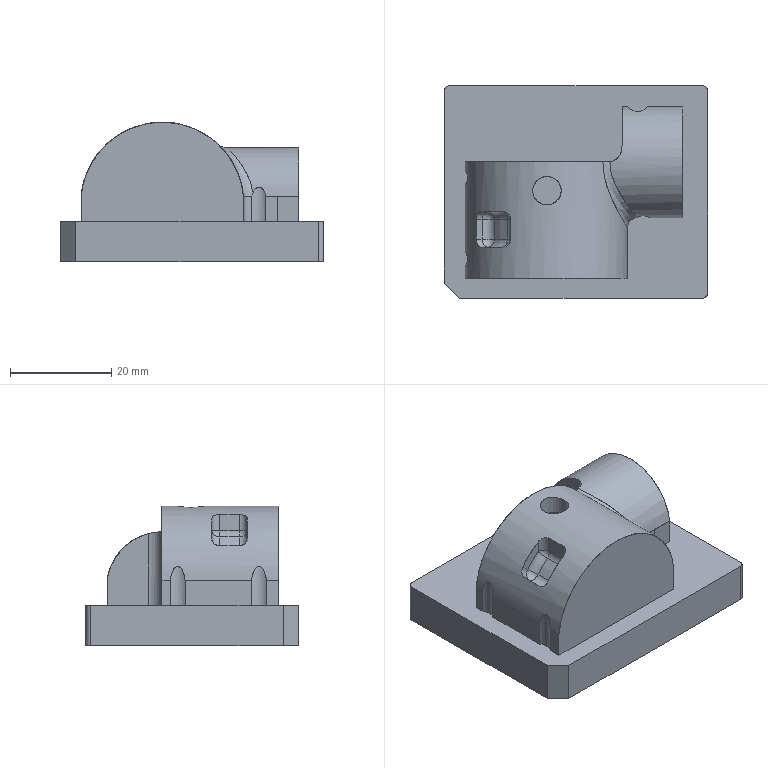NC program | PowerMill | posted with a generic post | part box 52 x 42 x 27.622 mm
Lines 34978 to 35880 of 322299:
N35075 M6
N35076 S8500 M03
N35077 G00 G90 X0.0 Y0.0
N35078 G43 Z9.8022 H3
N35079
N35080 G05 P10000 R8
N35081 X-31.8487 Y-27.3606
N35082 Z-18.62
N35083 G01 Z-19.82 F360.0
N35084 X-28.1181 Y-23.6313 F600.0
N35085 X-25.6571 Y-21.0381
N35086 X-25.7337 Y-20.9654
N35087 X-25.9275 Y-20.7611
N35088 G02 X-26.2819 Y-20.3235 I4.7332 J4.1953
N35089 G01 X-26.4415 Y-20.0914
N35090 X-26.5886 Y-19.8512
N35091 X-26.723 Y-19.6037
N35092 X-26.8443 Y-19.3494
N35093 X-26.9521 Y-19.0892
N35094 X-27.0461 Y-18.8237
N35095 X-27.1261 Y-18.5536
N35096 X-27.1919 Y-18.2798
N35097 X-27.2432 Y-18.0028
N35098 X-27.28 Y-17.7236
N35099 X-27.3021 Y-17.4428
N35100 X-27.3094 Y-17.1612
N35101 Y-14.7229
N35102 X-27.3036 Y-14.4732
N35103 X-27.2863 Y-14.2241
N35104 G02 X-27.2169 Y-13.7296 I6.013 J-0.5908
N35105 G01 X-27.1651 Y-13.4853
N35106 G03 Y-13.002 I-0.9704 J0.2416
N35107 G01 X-27.2169 Y-12.7577
N35108 G02 X-27.2836 Y-12.2858 I5.5385 J1.0235
N35109 G01 X-27.3036 Y-12.0141
N35110 X-27.3094 Y-11.7644
N35111 Y1.3491
N35112 X-27.3036 Y1.5988
N35113 X-27.2863 Y1.8479
N35114 X-27.2573 Y2.096
N35115 X-27.2169 Y2.3424
N35116 X-27.1652 Y2.5867
N35117 G03 X-27.1651 Y3.07 I-0.9703 J0.2417
N35118 G01 X-27.2169 Y3.3143
N35119 X-27.2574 Y3.5607
N35120 X-27.2863 Y3.8088
N35121 X-27.3036 Y4.0579
N35122 X-27.3094 Y4.3076
N35123 Y5.9414
N35124 X-27.3021 Y6.223
N35125 X-27.28 Y6.5038
N35126 X-27.2432 Y6.783
N35127 X-27.1919 Y7.06
N35128 G02 X-27.0461 Y7.6039 I6.0891 J-1.3403
N35129 G01 X-26.9521 Y7.8694
N35130 X-26.8443 Y8.1296
N35131 X-26.723 Y8.3839
N35132 X-26.5886 Y8.6314
N35133 X-26.4415 Y8.8716
N35134 X-26.2819 Y9.1037
N35135 X-26.1105 Y9.3271
N35136 X-25.9275 Y9.5413
N35137 X-25.7337 Y9.7456
N35138 G02 X-25.3152 Y10.1224 I4.4805 J-4.5554
N35139 G01 X-25.0917 Y10.2939
N35140 X-24.939 Y10.3996
N35141 X-24.6194 Y10.6006
N35142 G02 X-24.1177 Y10.8563 I3.1471 J-5.5562
N35143 G02 X-23.6375 Y11.0427 I2.5178 J-5.7736
N35144 G01 X-25.0116 Y15.6429
N35145 X-25.5677 Y15.4768
N35146 G02 X-26.6731 Y16.3431 I-0.2462 J0.8242
N35147 G01 X-26.5211 Y19.4408
N35148 G02 X-24.2089 Y21.645 I2.3149 J-0.1135
N35149 G01 X-1.0643 Y21.6726
N35150 G02 X-0.2545 Y20.5497 I0.001 J-0.8527
N35151 G01 X-0.3586 Y20.2381
N35152 G03 X-0.885 Y18.0053 I11.9898 J-4.0052
N35153 G01 X-0.9904 Y17.2609
N35154 G02 X-2.2961 Y16.1268 I-1.3061 J0.185
N35155 G01 X-21.9374 Y16.1214
N35156 G03 X-24.8262 Y15.6983 I0.0062 J-10.115
N35157 G01 X-25.0116 Y15.6429
N35158 X-23.6375 Y11.0427
N35159 X-23.5919 Y11.0581
N35160 G02 X-23.048 Y11.2038 I1.9409 J-6.1558
N35161 G02 X-22.4918 Y11.2919 I1.2833 J-6.3024
N35162 G02 X-21.9294 Y11.3214 I0.6203 J-6.4566
N35163 G01 X2.7714
N35164 G03 X3.7713 Y12.3039 I0.0 J1.0
N35165 G01 X3.8512 Y16.882
N35166 X3.8633 Y17.1603
N35167 X3.8897 Y17.4376
N35168 X3.9305 Y17.7131
N35169 G02 X4.0545 Y18.256 I6.1181 J-1.112
N35170 G01 X4.1374 Y18.5219
N35171 X4.234 Y18.7832
N35172 X4.3439 Y19.0391
N35173 X4.467 Y19.289
N35174 X4.6028 Y19.5322
N35175 X4.751 Y19.768
N35176 X4.9112 Y19.9958
N35177 X5.083 Y20.2151
N35178 X5.2659 Y20.4251
N35179 G02 X5.6631 Y20.8154 I4.6843 J-4.3696
N35180 G01 X5.8763 Y20.9947
N35181 G02 X6.3292 Y21.3188 I3.9432 J-5.0294
N35182 G02 X6.813 Y21.5945 I3.414 J-5.4309
N35183 G02 X7.3228 Y21.8186 I2.7941 J-5.6635
N35184 G01 X7.5857 Y21.9106
N35185 X7.853 Y21.9888
N35186 X8.124 Y22.0532
N35187 G02 X8.9519 Y22.1609 I1.153 J-5.6244
N35188 G01 X9.2304 Y22.1681
N35189 X10.276
N35190 X10.5574 Y22.1608
N35191 X10.8381 Y22.1387
N35192 X11.1172 Y22.102
N35193 X11.3941 Y22.0507
N35194 X11.6678 Y21.985
N35195 X11.9192 Y21.9105
N35196 G03 X12.4871 I0.284 J0.9589
N35197 G01 X12.7386 Y21.985
N35198 X13.0124 Y22.0507
N35199 G02 X13.5684 Y22.1387 I1.2893 J-6.3441
N35200 G01 X13.849 Y22.1608
N35201 X14.1305 Y22.1681
N35202 X21.0985
N35203 G02 X21.6609 Y22.1387 I-0.0522 J-6.3768
N35204 G01 X21.9401 Y22.1019
N35205 G02 X22.491 Y21.9848 I-1.0667 J-6.3733
N35206 G01 X22.761 Y21.9048
N35207 X23.0265 Y21.8108
N35208 X23.2868 Y21.703
N35209 X23.541 Y21.5818
N35210 X23.7885 Y21.4473
N35211 X24.0287 Y21.3002
N35212 X24.2608 Y21.1406
N35213 X24.4843 Y20.9692
N35214 X24.6984 Y20.7862
N35215 X24.9028 Y20.5924
N35216 X25.0967 Y20.3881
N35217 X25.2796 Y20.1739
N35218 G02 X25.6106 Y19.7183 I-5.0349 J-4.0059
N35219 G01 X25.7578 Y19.4781
N35220 G02 X26.0134 Y18.9764 I-5.3387 J-3.0361
N35221 G01 X26.1212 Y18.7162
N35222 X26.2152 Y18.4506
N35223 X26.2952 Y18.1806
N35224 G02 X26.4123 Y17.6297 I-6.1271 J-1.5904
N35225 G01 X26.4491 Y17.3505
N35226 X26.4712 Y17.0697
N35227 X26.4785 Y16.7881
N35228 Y-5.1044
N35229 X26.4712 Y-5.386
N35230 G02 X26.4123 Y-5.9461 I-6.3455 J0.384
N35231 G01 X26.361 Y-6.223
N35232 X26.2952 Y-6.4969
N35233 G02 X26.1212 Y-7.0325 I-6.0528 J1.6708
N35234 G01 X26.0134 Y-7.2927
N35235 X25.8921 Y-7.5469
N35236 G02 X25.6106 Y-8.0346 I-5.4965 J2.8484
N35237 G01 X25.451 Y-8.2667
N35238 X25.2796 Y-8.4902
N35239 X25.0966 Y-8.7044
N35240 X24.9028 Y-8.9087
N35241 X24.6609 Y-9.1346
N35242 X24.4843 Y-9.2855
N35243 X24.2608 Y-9.457
N35244 X24.0287 Y-9.6165
N35245 G02 X23.541 Y-9.898 I-3.4798 J5.4641
N35246 G01 X23.3637 Y-9.9833
N35247 X23.1837 Y-10.063
N35248 X24.9739 Y-14.5121
N35249 X25.5789 Y-14.2687
N35250 G02 X26.672 Y-15.0123 I0.2972 J-0.7384
N35251 G01 X26.6451 Y-19.12
N35252 G02 X24.1039 Y-21.6553 I-2.5521 J0.0168
N35253 G01 X20.6535 Y-21.6699
N35254 G02 X19.7994 Y-20.5579 I-0.0038 J0.8811
N35255 G01 X20.015 Y-19.7638
N35256 G03 X20.4201 Y-16.8462 I-11.2116 J3.0438
N35257 G01 X20.4236 Y-16.5257
N35258 G02 X21.4806 Y-15.3283 I1.2218 J-0.0133
N35259 G01 X22.4201 Y-15.2004
N35260 G03 X24.8875 Y-14.5469 I-1.3955 J10.2539
N35261 G01 X24.9739 Y-14.5121
N35262 X23.1837 Y-10.063
N35263 X23.0265 Y-10.1271
N35264 G02 X22.491 Y-10.3011 I-2.2591 J6.0418
N35265 G01 X22.2171 Y-10.3669
N35266 G02 X21.6609 Y-10.455 I-1.2851 J6.3138
N35267 G01 X21.3801 Y-10.4771
N35268 X21.0985 Y-10.4844
N35269 X16.5539
N35270 G03 X15.5539 Y-11.4844 I0.0 J-1.0
N35271 G01 Y-17.1612
N35272 G02 X15.5244 Y-17.7236 I-6.4151 J0.0544
N35273 G01 X15.4877 Y-18.0028
N35274 X15.4363 Y-18.2798
N35275 G02 X15.2906 Y-18.8237 I-6.2037 J1.3709
N35276 G01 X15.1966 Y-19.0892
N35277 X15.0888 Y-19.3494
N35278 G02 X14.8331 Y-19.8512 I-5.7149 J2.5959
N35279 G01 X14.6859 Y-20.0914
N35280 X14.5264 Y-20.3235
N35281 X14.3549 Y-20.547
N35282 X14.172 Y-20.7611
N35283 X13.9511 Y-20.9911
N35284 X13.7738 Y-21.1593
N35285 X13.5596 Y-21.3423
N35286 X13.3362 Y-21.5137
N35287 G02 X12.8011 Y-21.8545 I-3.2487 J4.5101
N35288 G01 X12.6164 Y-21.9548
N35289 G02 X12.1019 Y-22.1839 I-2.856 J5.7221
N35290 G01 X11.8364 Y-22.2779
N35291 X11.5663 Y-22.3579
N35292 G02 X11.0155 Y-22.475 I-1.6116 J6.2279
N35293 G01 X10.7362 Y-22.5117
N35294 X10.4554 Y-22.5338
N35295 X10.1739 Y-22.5412
N35296 X-21.9294
N35297 X-22.211 Y-22.5338
N35298 X-22.4918 Y-22.5117
N35299 X-22.7711 Y-22.475
N35300 X-23.048 Y-22.4236
N35301 G02 X-23.592 Y-22.2779 I1.3914 J6.2809
N35302 G02 X-24.1177 Y-22.0761 I2.0424 J6.106
N35303 G02 X-24.6194 Y-21.8204 I2.6836 J5.887
N35304 G01 X-24.867 Y-21.6684
N35305 X-25.0917 Y-21.5137
N35306 X-25.3152 Y-21.3422
N35307 X-25.5294 Y-21.1593
N35308 X-25.6571 Y-21.0381
N35309 X-28.1181 Y-23.6313
N35310 G00 Z9.8022
N35311 G05 P0
N35312 (---------------)
N35313 ( END TOOLPATH : 精公基准台01-基准面偏置-D10 )
N35314 (---------------)
N35315 ( START TOOLPATH : 精公基准台01-外形侧光-D10 )
N35316 (---------------)
N35317 G00 X0.0 Y0.0 Z10.802
N35318 G05 P10000 R8
N35319 X-22.6288 Y11.0478
N35320 Z-8.294
N35321 G01 Z-9.494 F360.0
N35322 G03 X-21.4997 Y10.8403 I0.815 J1.2593 F600.0
N35323 G02 X-20.4463 Y10.9514 I1.0491 J-4.899
N35324 G01 X3.9012
N35325 G03 X4.1212 Y11.1676 I0.0 J0.22
N35326 G01 X4.1792 Y14.5154
N35327 G02 X4.3087 Y15.6056 I5.0106 J-0.0423
N35328 G03 X4.1205 Y16.7381 I-1.4612 J0.3391
N35329 G00 Z4.0256
N35330 G01 X26.2065 Y16.6492 F10000.0
N35331 G00 Z-8.294
N35332 G01 Z-9.494 F360.0
N35333 G03 X25.9982 Y15.5203 I1.2587 J-0.8159 F600.0
N35334 G02 X26.1084 Y14.5132 I-4.8997 J-1.0455
N35335 G01 X26.1083 Y-2.8318
N35336 G02 X25.9992 Y-3.832 I-5.01 J0.0407
N35337 G03 X26.2086 Y-4.9608 I1.4672 J-0.3116
N35338 G00 Z4.0256
N35339 G01 X10.8659 Y-22.2707 F10000.0
N35340 G00 Z-8.294
N35341 G01 Z-9.494 F360.0
N35342 G03 X9.7371 Y-22.0616 I-0.8168 J-1.2581 F600.0
N35343 G02 X8.7627 Y-22.1707 I-1.0422 J4.9005
N35344 G01 X-5.9331 Y-22.171
N35345 X-20.4477 Y-22.1712
N35346 G02 X-21.4998 Y-22.0601 I-0.0028 J5.0101
N35347 G03 X-22.629 Y-22.2675 I-0.3142 J-1.4667
N35348 G00 Z4.0256
N35349 G01 X-22.1045 Y11.1586 F10000.0
N35350 G00 Z-8.294
N35351 G01 Z-9.494 F360.0
N35352 G03 X-21.0014 Y10.8405 I0.9355 J1.1725 F600.0
N35353 G02 X-20.4464 Y10.8714 I0.5509 J-4.8994
N35354 G01 X-20.4463
N35355 X3.9012
N35356 G03 X4.2012 Y11.1662 I0.0 J0.3
N35357 G01 X4.2592 Y14.5132
N35358 G02 X4.3 Y15.1075 I4.9305 J-0.0401
N35359 G03 X4.0008 Y16.2159 I-1.4875 J0.193
N35360 G00 Z4.0256
N35361 G01 X26.3175 Y16.1231 F10000.0
N35362 G00 Z-8.294
N35363 G01 Z-9.494 F360.0
N35364 G03 X25.9982 Y15.0203 I1.1715 J-0.9368 F600.0
N35365 G02 X26.0284 Y14.5132 I-4.8991 J-0.5455
N35366 G01 Y-2.8296
N35367 G02 X25.9991 Y-3.3283 I-4.9304 J0.0385
N35368 G03 X26.3203 Y-4.4305 I1.4911 J-0.1635
N35369 G00 Z4.0256
N35370 G01 X10.3369 Y-22.3822 F10000.0
N35371 G00 Z-8.294
N35372 G01 Z-9.494 F360.0
N35373 G03 X9.2345 Y-22.0616 I-0.9382 J-1.1703 F600.0
N35374 G02 X8.7627 Y-22.0907 I-0.5396 J4.9001
N35375 G01 X-5.9331 Y-22.0912
N35376 X-20.4463
N35377 G02 X-21.0034 Y-22.0601 I-0.0042 J4.9299
N35378 G03 X-22.1067 Y-22.3777 I-0.1683 J-1.4905
N35379 G00 Z3.8883
N35380 G01 X15.6233 Y-12.1522 F10000.0
N35381 G00 Z-18.59
N35382 G01 Z-19.79 F360.0
N35383 G03 X15.1839 Y-13.2128 I1.0606 J-1.0606 F600.0
N35384 G01 Y-17.0694
N35385 G02 X10.2232 Y-22.171 I-5.0119 J-0.0892
N35386 G01 X-5.9331 Y-22.1711
N35387 X-21.0034 Y-22.1712
N35388 X-21.9079
N35389 G02 X-26.9386 Y-17.2516 I-0.0214 J5.0101
N35390 G01 X-26.9393 Y-14.6939
N35391 G02 X-26.7343 Y-13.307 I4.93 J-0.0202
N35392 G03 X-26.7338 Y-13.1846 I-0.2111 J0.0622
N35393 G02 X-26.9394 Y-11.7749 I4.7923 J1.419
N35394 G01 Y1.371
N35395 G02 X-26.7342 Y2.7679 I4.9962 J-0.0204
N35396 G03 Y2.8887 I-0.2115 J0.0605
N35397 G02 X-26.9394 Y4.2901 I4.7926 J1.4177
N35398 G01 Y5.9344
N35399 G02 X-21.9068 Y10.9514 I5.0102 J0.0068
N35400 G01 X-20.4464
N35401 X3.9013
N35402 G03 X4.116 Y11.1237 I0.0 J0.22
N35403 G03 X4.1212 Y11.1676 I-0.2148 J0.0477
N35404 G01 X4.2214 Y16.8895
N35405 G02 X9.3104 Y21.7981 I5.011 J-0.1028
N35406 G02 X10.4093 Y21.7964 I0.4565 J-57.2258
N35407 G02 X12.1216 Y21.4452 I-0.123 J-4.9497
N35408 G03 X12.2855 Y21.4447 I0.0826 J0.2039
N35409 G02 X14.0568 Y21.7976 I1.8327 J-4.5763
N35410 G01 X21.1793 Y21.7975
N35411 G02 X26.1085 Y16.7039 I-0.0824 J-5.0116
N35412 G01 Y-5.0207
N35413 G02 X21.1765 Y-10.1138 I-5.0115 J-0.0815
N35414 G01 X15.4039 Y-10.1144
N35415 G03 X15.1839 Y-10.3344 I0.0 J-0.22
N35416 G01 Y-13.2128
N35417 G03 X15.6232 Y-14.2735 I1.5 J0.0
N35418 G01 X15.5433 Y-12.0854
N35419 G03 X15.1039 Y-13.146 I1.0606 J-1.0606
N35420 G01 Y-17.069
N35421 G02 X10.2232 Y-22.091 I-4.9319 J-0.0896
N35422 G01 X-5.9331 Y-22.0912
N35423 X-21.0034
N35424 X-21.9068
N35425 G02 X-26.8586 Y-17.2516 I-0.0225 J4.9301
N35426 G02 X-26.8594 Y-14.6958 I279.1536 J1.3602
N35427 G02 X-26.6576 Y-13.3296 I4.85 J-0.0183
N35428 G03 X-26.6568 Y-13.1627 I-0.2878 J0.0848
N35429 G02 X-26.8594 Y-11.7749 I4.7132 J1.3968
N35430 G01 Y1.3692
N35431 G02 X-26.6573 Y2.7459 I4.9162 J-0.0186
N35432 G03 X-26.6572 Y2.9107 I-0.2884 J0.0825
N35433 G02 X-26.8594 Y4.2901 I4.7139 J1.3954
N35434 G01 Y5.9331
N35435 G02 X-21.9068 Y10.8714 I4.9301 J0.0082
N35436 G01 X-20.4464
N35437 X3.9013
N35438 G03 X4.1941 Y11.1063 I0.0 J0.3
N35439 G03 X4.2012 Y11.1662 I-0.2929 J0.0651
N35440 G01 X4.3013 Y16.8865
N35441 G02 X9.3104 Y21.7181 I4.9311 J-0.0998
N35442 G02 X10.4057 Y21.7164 I0.4564 J-58.6332
N35443 G02 X12.0916 Y21.371 I-0.1194 J-4.8696
N35444 G03 X12.3151 Y21.3703 I0.1126 J0.2781
N35445 G02 X14.0568 Y21.7176 I1.8029 J-4.5009
N35446 G01 X21.1765 Y21.7175
N35447 G02 X26.0285 Y16.7039 I-0.0796 J-4.9316
N35448 G01 Y-5.0203
N35449 G02 X21.1765 Y-10.0338 I-4.9315 J-0.0819
N35450 G01 X15.4039 Y-10.0344
N35451 G03 X15.1039 Y-10.3344 I0.0 J-0.3
N35452 G01 Y-13.146
N35453 G03 X15.5432 Y-14.2067 I1.5 J0.0
N35454 G00 Z10.802
N35455 G05 P0
N35456 (---------------)
N35457 ( END TOOLPATH : 精公基准台01-外形侧光-D10 )
N35458 (---------------)
N35459 ( START TOOLPATH : 精公基准台01-基准台侧光-D10 )
N35460 (---------------)
N35461 G00 X0.0 Y0.0 Z9.8022
N35462 G05 P10000 R8
N35463 X31.3451 Y-29.0791
N35464 Z-26.52
N35465 G01 Z-27.72 F360.0
N35466 G03 X28.4718 Y-24.9872 I-1.4367 J2.0459 F600.0
N35467 G01 X28.341 Y-25.079
N35468 X28.3395 Y-25.0801
N35469 X28.3379 Y-25.0811
N35470 X28.1487 Y-25.2011
N35471 X28.1476 Y-25.2018
N35472 X28.1464 Y-25.2025
N35473 X28.0195 Y-25.2772
N35474 X28.018 Y-25.2781
N35475 X28.0165 Y-25.2789
N35476 X27.7004 Y-25.4474
N35477 X27.6988 Y-25.4482
N35478 X27.6972 Y-25.449
N35479 X27.5446 Y-25.5219
N35480 X27.5435 Y-25.5224
N35481 X27.5424 Y-25.5229
N35482 X27.379 Y-25.5952
N35483 X27.3774 Y-25.5959
N35484 X27.3758 Y-25.5965
N35485 X27.0597 Y-25.7205
N35486 X27.0574 Y-25.7213
N35487 X27.0551 Y-25.7221
N35488 X26.6842 Y-25.842
N35489 X26.6821 Y-25.8426
N35490 X26.68 Y-25.8432
N35491 X26.4186 Y-25.9122
N35492 X26.4166 Y-25.9127
N35493 X26.4146 Y-25.9131
N35494 X26.0984 Y-25.9794
N35495 X26.0965 Y-25.9798
N35496 X26.0945 Y-25.9802
N35497 X25.7783 Y-26.03
N35498 X25.7761 Y-26.0303
N35499 X25.7739 Y-26.0305
N35500 X25.4577 Y-26.0623
N35501 X25.4557 Y-26.0624
N35502 X25.4537 Y-26.0626
N35503 X25.1375 Y-26.0781
N35504 X25.1358 Y-26.0782
N35505 X25.134
N35506 X24.8179 Y-26.08
N35507 X24.8177
N35508 X24.8174
N35509 X-22.9206
N35510 X-22.9213
N35511 X-22.922
N35512 X-23.2381 Y-26.0744
N35513 X-23.2406 Y-26.0743
N35514 X-23.243 Y-26.0742
N35515 X-23.5592 Y-26.0491
N35516 X-23.5617 Y-26.0489
N35517 X-23.5642 Y-26.0485
N35518 X-23.8804 Y-26.0031
N35519 X-23.8829 Y-26.0027
N35520 X-23.8854 Y-26.0022
N35521 X-24.2016 Y-25.9358
N35522 X-24.2041 Y-25.9352
N35523 X-24.2066 Y-25.9346
N35524 X-24.5228 Y-25.8464
N35525 X-24.5253 Y-25.8456
N35526 X-24.5279 Y-25.8448
N35527 X-24.844 Y-25.7335
N35528 X-24.8465 Y-25.7325
N35529 X-24.8491 Y-25.7315
N35530 X-25.1652 Y-25.5954
N35531 X-25.1671 Y-25.5946
N35532 X-25.1689 Y-25.5937
N35533 X-25.3157 Y-25.5215
N35534 X-25.3169 Y-25.5209
N35535 X-25.3182 Y-25.5202
N35536 X-25.4876 Y-25.4293
N35537 X-25.4895 Y-25.4282
N35538 X-25.4915 Y-25.427
N35539 X-25.8076 Y-25.2336
N35540 X-25.8102 Y-25.2319
N35541 X-25.8127 Y-25.2302
N35542 X-26.1288 Y-25.002
N35543 X-26.1307 Y-25.0006
N35544 X-26.1325 Y-24.9992
N35545 X-26.2796 Y-24.8795
N35546 X-26.2809 Y-24.8784
N35547 X-26.2822 Y-24.8773
N35548 X-26.4512 Y-24.7277
N35549 X-26.4525 Y-24.7264
N35550 X-26.4539 Y-24.7252
N35551 X-26.6255 Y-24.5587
N35552 X-26.6259 Y-24.5583
N35553 X-26.6264 Y-24.5579
N35554 X-29.6162 Y-21.5679
N35555 X-29.617 Y-21.567
N35556 X-29.6179 Y-21.5661
N35557 X-29.7792 Y-21.3947
N35558 X-29.7805 Y-21.3933
N35559 X-29.7818 Y-21.3918
N35560 X-29.9366 Y-21.2109
N35561 X-29.9376 Y-21.2096
N35562 X-29.9386 Y-21.2083
N35563 X-30.045 Y-21.0732
N35564 X-30.0463 Y-21.0715
N35565 X-30.0476 Y-21.0697
N35566 X-30.2573 Y-20.7714
N35567 X-30.259 Y-20.7689
N35568 X-30.2606 Y-20.7664
N35569 X-30.4598 Y-20.4324
N35570 X-30.4612 Y-20.4298
N35571 X-30.4626 Y-20.4272
N35572 X-30.6206 Y-20.111
N35573 X-30.6218 Y-20.1085
N35574 X-30.6229 Y-20.1059
N35575 X-30.7542 Y-19.7898
N35576 X-30.7552 Y-19.7873
N35577 X-30.7561 Y-19.7847
N35578 X-30.863 Y-19.4686
N35579 X-30.8636 Y-19.4668
N35580 X-30.8642 Y-19.465
N35581 X-30.9011 Y-19.3363
N35582 X-30.9015 Y-19.335
N35583 X-30.9018 Y-19.3337
N35584 X-30.949 Y-19.1463
N35585 X-30.9494 Y-19.1443
N35586 X-30.9499 Y-19.1423
N35587 X-31.0123 Y-18.8262
N35588 X-31.0128 Y-18.8237
N35589 X-31.0132 Y-18.8211
N35590 X-31.0548 Y-18.505
N35591 X-31.0551 Y-18.5024
N35592 X-31.0553 Y-18.4999
N35593 X-31.0766 Y-18.1838
N35594 X-31.0768 Y-18.1815
N35595 Y-18.1792
N35596 X-31.08 Y-17.863
N35597 Y-17.8626
N35598 Y-17.8622
N35599 X-31.0794 Y20.0753
N35600 Y20.0768
N35601 Y20.0783
N35602 X-31.0672 Y20.3945
N35603 X-31.0671 Y20.3966
N35604 X-31.0669 Y20.3987
N35605 X-31.0377 Y20.7149
N35606 X-31.0375 Y20.717
N35607 X-31.0372 Y20.7191
N35608 X-30.9912 Y21.0352
N35609 X-30.9908 Y21.0373
N35610 X-30.9904 Y21.0395
N35611 X-30.9269 Y21.3556
N35612 X-30.9264 Y21.3577
N35613 X-30.9259 Y21.3598
N35614 X-30.8443 Y21.676
N35615 X-30.8437 Y21.6781
N35616 X-30.8431 Y21.6802
N35617 X-30.7428 Y21.9963
N35618 X-30.7421 Y21.9984
N35619 X-30.7413 Y22.0005
N35620 X-30.6213 Y22.3167
N35621 X-30.6205 Y22.3188
N35622 X-30.6195 Y22.3209
N35623 X-30.4782 Y22.6371
N35624 X-30.4772 Y22.6392
N35625 X-30.4761 Y22.6413
N35626 X-30.3121 Y22.9574
N35627 X-30.3109 Y22.9595
N35628 X-30.3097 Y22.9616
N35629 X-30.1205 Y23.2778
N35630 X-30.1192 Y23.2799
N35631 X-30.1178 Y23.282
N35632 X-29.901 Y23.5981
N35633 X-29.8993 Y23.6004
N35634 X-29.8977 Y23.6026
N35635 X-29.6223 Y23.9496
N35636 X-29.6204 Y23.952
N35637 X-29.6184 Y23.9542
N35638 X-29.3022 Y24.2961
N35639 X-29.3003 Y24.2982
N35640 X-29.2982 Y24.3002
N35641 X-29.0218 Y24.5596
N35642 X-29.0198 Y24.5615
N35643 X-29.0176 Y24.5633
N35644 X-28.6617 Y24.8535
N35645 X-28.6595 Y24.8553
N35646 X-28.6572 Y24.857
N35647 X-28.341 Y25.079
N35648 X-28.3395 Y25.0801
N35649 X-28.3379 Y25.0811
N35650 X-28.1487 Y25.2011
N35651 X-28.1476 Y25.2018
N35652 X-28.1464 Y25.2025
N35653 X-28.0195 Y25.2772
N35654 X-28.018 Y25.2781
N35655 X-28.0165 Y25.2789
N35656 X-27.7004 Y25.4474
N35657 X-27.6988 Y25.4482
N35658 X-27.6972 Y25.449
N35659 X-27.5446 Y25.5219
N35660 X-27.5435 Y25.5224
N35661 X-27.5424 Y25.5229
N35662 X-27.379 Y25.5952
N35663 X-27.3774 Y25.5959
N35664 X-27.3758 Y25.5965
N35665 X-27.0597 Y25.7205
N35666 X-27.0576 Y25.7213
N35667 X-27.0554 Y25.722
N35668 X-26.7393 Y25.8259
N35669 X-26.7372 Y25.8265
N35670 X-26.7351 Y25.8271
N35671 X-26.4189 Y25.9121
N35672 X-26.4168 Y25.9126
N35673 X-26.4146 Y25.9131
N35674 X-26.0984 Y25.9795
N35675 X-26.0965 Y25.9798
N35676 X-26.0945 Y25.9802
N35677 X-25.7783 Y26.0299
N35678 X-25.7761 Y26.0303
N35679 X-25.7739 Y26.0305
N35680 X-25.4577 Y26.0623
N35681 X-25.4557 Y26.0624
N35682 X-25.4537 Y26.0626
N35683 X-25.1375 Y26.0781
N35684 X-25.1358 Y26.0782
N35685 X-25.134
N35686 X-24.8179 Y26.08
N35687 X-24.8177
N35688 X-24.8174
N35689 X0.0
N35690 X24.8174
N35691 X24.8177
N35692 X24.8179
N35693 X25.134 Y26.0782
N35694 X25.1357
N35695 X25.1374 Y26.0781
N35696 X25.4535 Y26.063
N35697 X25.4557 Y26.0629
N35698 X25.4578 Y26.0627
N35699 X25.774 Y26.0305
N35700 X25.7761 Y26.0303
N35701 X25.7782 Y26.03
N35702 X26.0943 Y25.9807
N35703 X26.0965 Y25.9803
N35704 X26.0986 Y25.9799
N35705 X26.4147 Y25.9131
N35706 X26.4166 Y25.9127
N35707 X26.4186 Y25.9122
N35708 X26.6797 Y25.8432
N35709 X26.6819 Y25.8426
N35710 X26.684 Y25.842
N35711 X27.0551 Y25.7217
N35712 X27.0574 Y25.721
N35713 X27.0596 Y25.7201
N35714 X27.3757 Y25.5966
N35715 X27.3774 Y25.5959
N35716 X27.379 Y25.5952
N35717 X27.5424 Y25.5229
N35718 X27.5436 Y25.5224
N35719 X27.5447 Y25.5218
N35720 X27.6974 Y25.4484
N35721 X27.6989 Y25.4477
N35722 X27.7003 Y25.447
N35723 X28.0164 Y25.2789
N35724 X28.018 Y25.2781
N35725 X28.0195 Y25.2772
N35726 X28.1464 Y25.2025
N35727 X28.1475 Y25.2019
N35728 X28.1485 Y25.2012
N35729 X28.3377 Y25.0819
N35730 X28.3393 Y25.0809
N35731 X28.3409 Y25.0798
N35732 X28.6224 Y24.883
N35733 X28.6245 Y24.8815
N35734 X28.6266 Y24.8798
N35735 X28.9774 Y24.5985
N35736 X28.9796 Y24.5966
N35737 X28.9818 Y24.5946
N35738 X29.298 Y24.3004
N35739 X29.2993 Y24.2992
N35740 X29.3005 Y24.2979
N35741 X29.3563 Y24.2412
N35742 X29.3573 Y24.2401
N35743 X29.3584 Y24.239
N35744 X29.6188 Y23.9533
N35745 X29.6205 Y23.9512
N35746 X29.6223 Y23.9492
N35747 X29.8976 Y23.6026
N35748 X29.8993 Y23.6004
N35749 X29.901 Y23.5981
N35750 X30.1178 Y23.282
N35751 X30.1192 Y23.2799
N35752 X30.1205 Y23.2778
N35753 X30.3097 Y22.9616
N35754 X30.3109 Y22.9596
N35755 X30.312 Y22.9574
N35756 X30.4763 Y22.6413
N35757 X30.4773 Y22.6392
N35758 X30.4783 Y22.637
N35759 X30.6196 Y22.3209
N35760 X30.6205 Y22.3188
N35761 X30.6213 Y22.3167
N35762 X30.7414 Y22.0005
N35763 X30.7422 Y21.9984
N35764 X30.7429 Y21.9963
N35765 X30.8432 Y21.6802
N35766 X30.8438 Y21.6781
N35767 X30.8444 Y21.676
N35768 X30.926 Y21.3598
N35769 X30.9265 Y21.3576
N35770 X30.927 Y21.3554
N35771 X30.9897 Y21.0393
N35772 X30.9901 Y21.0373
N35773 X30.9904 Y21.0354
N35774 X31.0372 Y20.7193
N35775 X31.0375 Y20.717
N35776 X31.0377 Y20.7147
N35777 X31.066 Y20.3985
N35778 X31.0662 Y20.3966
N35779 X31.0663 Y20.3947
N35780 X31.0794 Y20.0786
N35781 Y20.0769
N35782 Y20.0753
N35783 Y-20.0753
N35784 Y-20.0768
N35785 Y-20.0783
N35786 X31.0672 Y-20.3945
N35787 X31.0671 Y-20.3966
N35788 X31.0669 Y-20.3987
N35789 X31.0377 Y-20.7149
N35790 X31.0375 Y-20.717
N35791 X31.0372 Y-20.7191
N35792 X30.9912 Y-21.0352
N35793 X30.9909 Y-21.0373
N35794 X30.9905 Y-21.0395
N35795 X30.9269 Y-21.3556
N35796 X30.9264 Y-21.3577
N35797 X30.9259 Y-21.3598
N35798 X30.8443 Y-21.676
N35799 X30.8437 Y-21.6781
N35800 X30.8431 Y-21.6802
N35801 X30.7428 Y-21.9963
N35802 X30.7421 Y-21.9984
N35803 X30.7413 Y-22.0005
N35804 X30.6213 Y-22.3167
N35805 X30.6205 Y-22.3188
N35806 X30.6195 Y-22.3209
N35807 X30.4782 Y-22.6371
N35808 X30.4772 Y-22.6392
N35809 X30.4761 Y-22.6413
N35810 X30.3121 Y-22.9574
N35811 X30.3109 Y-22.9595
N35812 X30.3097 Y-22.9616
N35813 X30.1205 Y-23.2778
N35814 X30.1192 Y-23.2799
N35815 X30.1178 Y-23.282
N35816 X29.901 Y-23.5981
N35817 X29.8993 Y-23.6004
N35818 X29.8977 Y-23.6026
N35819 X29.6223 Y-23.9496
N35820 X29.6204 Y-23.952
N35821 X29.6184 Y-23.9542
N35822 X29.3022 Y-24.2961
N35823 X29.3003 Y-24.2982
N35824 X29.2982 Y-24.3002
N35825 X29.0218 Y-24.5596
N35826 X29.0198 Y-24.5615
N35827 X29.0176 Y-24.5633
N35828 X28.6617 Y-24.8535
N35829 X28.6595 Y-24.8553
N35830 X28.6572 Y-24.857
N35831 X28.4718 Y-24.9872
N35832 G03 X31.345 Y-29.0792 I1.4366 J-2.046
N35833 G01 X31.2937 Y-29.0175
N35834 G03 X28.4204 Y-24.9255 I-1.4366 J2.046
N35835 G01 X28.295 Y-25.0135
N35836 X28.1058 Y-25.1336
N35837 X27.9789 Y-25.2083
N35838 X27.6627 Y-25.3768
N35839 X27.5101 Y-25.4497
N35840 X27.3466 Y-25.522
N35841 X27.0305 Y-25.646
N35842 X26.6596 Y-25.7659
N35843 X26.3982 Y-25.8348
N35844 X26.082 Y-25.9012
N35845 X25.7659 Y-25.9509
N35846 X25.4497 Y-25.9827
N35847 X25.1336 Y-25.9982
N35848 X24.8174 Y-26.0
N35849 X-22.9206
N35850 X-23.2367 Y-25.9944
N35851 X-23.5529 Y-25.9694
N35852 X-23.869 Y-25.9239
N35853 X-24.1851 Y-25.8575
N35854 X-24.5013 Y-25.7693
N35855 X-24.8174 Y-25.658
N35856 X-25.1336 Y-25.5219
N35857 X-25.2803 Y-25.4497
N35858 X-25.4497 Y-25.3588
N35859 X-25.7659 Y-25.1653
N35860 X-26.082 Y-24.9372
N35861 X-26.2291 Y-24.8174
N35862 X-26.3982 Y-24.6678
N35863 X-26.5698 Y-24.5013
N35864 X-29.5596 Y-21.5113
N35865 X-29.721 Y-21.3398
N35866 X-29.8758 Y-21.1589
N35867 X-29.9821 Y-21.0237
N35868 X-30.1919 Y-20.7254
N35869 X-30.391 Y-20.3914
N35870 X-30.549 Y-20.0753
N35871 X-30.6803 Y-19.7591
N35872 X-30.7873 Y-19.443
N35873 X-30.8242 Y-19.3142
N35874 X-30.8714 Y-19.1268
N35875 X-30.9339 Y-18.8107
N35876 X-30.9755 Y-18.4945
N35877 X-30.9968 Y-18.1784
N35878 X-31.0 Y-17.8622
N35879 Y19.1268
N35880 X-30.9994 Y20.0753
N35881 X-30.9872 Y20.3914
N35882 X-30.9581 Y20.7075
N35883 X-30.912 Y21.0237
N35884 X-30.8484 Y21.3398
N35885 X-30.7668 Y21.656
N35886 X-30.6665 Y21.9721
N35887 X-30.5465 Y22.2883
N35888 X-30.4051 Y22.6044
N35889 X-30.2411 Y22.9206
N35890 X-30.0518 Y23.2367
N35891 X-29.835 Y23.5529
N35892 X-29.5596 Y23.8999
N35893 X-29.2435 Y24.2418
N35894 X-28.9671 Y24.5013
N35895 X-28.6112 Y24.7916
N35896 X-28.295 Y25.0135
N35897 X-28.1058 Y25.1336
N35898 X-27.9789 Y25.2083
N35899 X-27.6627 Y25.3768
N35900 X-27.5101 Y25.4497
N35901 X-27.3466 Y25.522
N35902 X-27.0305 Y25.646
N35903 X-26.7143 Y25.7499
N35904 X-26.3982 Y25.8348
N35905 X-26.082 Y25.9012
N35906 X-25.7659 Y25.9509
N35907 X-25.4497 Y25.9827
N35908 X-25.1336 Y25.9982
N35909 X-24.8174 Y26.0
N35910 X0.0
N35911 X24.8174
N35912 X25.1336 Y25.9982
N35913 X25.4497 Y25.9831
N35914 X25.7659 Y25.9509
N35915 X26.082 Y25.9016
N35916 X26.3982 Y25.8348
N35917 X26.6593 Y25.7659
N35918 X27.0305 Y25.6456
N35919 X27.3466 Y25.522
N35920 X27.5101 Y25.4497
N35921 X27.6627 Y25.3763
N35922 X27.9789 Y25.2083
N35923 X28.1058 Y25.1336
N35924 X28.295 Y25.0142
N35925 X28.5765 Y24.8174
N35926 X28.9273 Y24.5361
N35927 X29.2435 Y24.2418
N35928 X29.2992 Y24.1851
N35929 X29.5596 Y23.8994
N35930 X29.835 Y23.5529
N35931 X30.0518 Y23.2367
N35932 X30.2411 Y22.9206
N35933 X30.4053 Y22.6044
N35934 X30.5465 Y22.2883
N35935 X30.6666 Y21.9721
N35936 X30.7669 Y21.656
N35937 X30.8485 Y21.3398
N35938 X30.9113 Y21.0237
N35939 X30.9581 Y20.7075
N35940 X30.9864 Y20.3914
N35941 X30.9994 Y20.0753
N35942 X31.0 Y19.7591
N35943 Y-19.1268
N35944 X30.9994 Y-20.0753
N35945 X30.9872 Y-20.3914
N35946 X30.958 Y-20.7075
N35947 X30.912 Y-21.0237
N35948 X30.8484 Y-21.3398
N35949 X30.7668 Y-21.656
N35950 X30.6665 Y-21.9721
N35951 X30.5465 Y-22.2883
N35952 X30.4051 Y-22.6044
N35953 X30.2411 Y-22.9206
N35954 X30.0518 Y-23.2367
N35955 X29.835 Y-23.5529
N35956 X29.5596 Y-23.8999
N35957 X29.2435 Y-24.2418
N35958 X28.9671 Y-24.5013
N35959 X28.6112 Y-24.7916
N35960 X28.4204 Y-24.9255
N35961 G03 X31.2937 Y-29.0175 I1.4366 J-2.046
N35962 G00 Z9.8022
N35963 G05 P0
N35964 (---------------)
N35965 ( END TOOLPATH : 精公基准台01-基准台侧光-D10 )
N35966 (---------------)
N35967
N35968 M05
N35969 G53 Z0.0
N35970 (---------------)
N35971 ( START TOOLPATH : 精公精光01-平行-R2 )
N35972 (---------------)
N35973 ( TOOL NO.    :7 )
N35974 ( TOOL TYPE   : BALLNOSED)
N35975 ( TOOL ID     : R2_1_1)
N35976 ( TOOL DIA    : 4.0 LENGTH 71.76)
N35977 T7